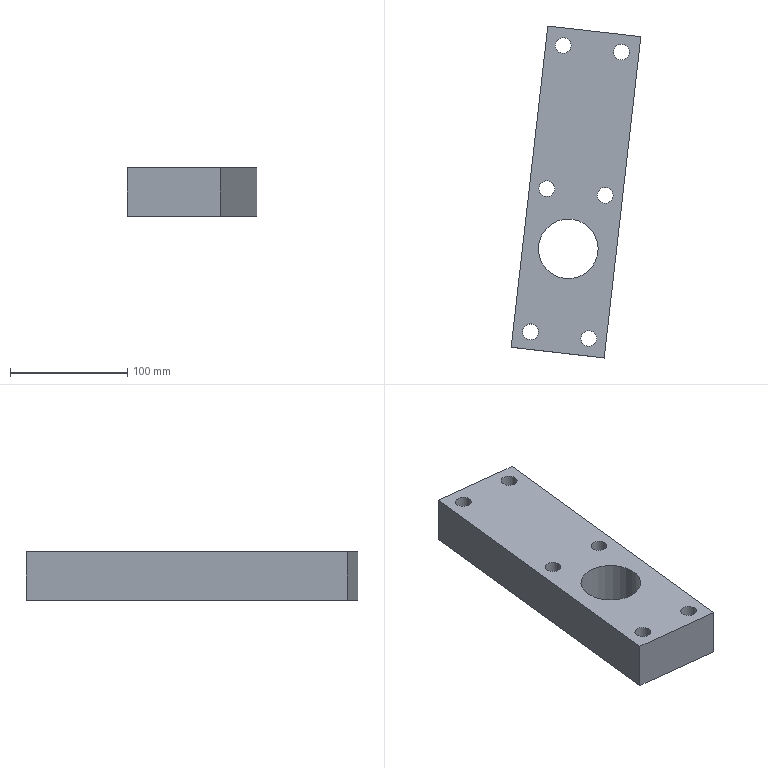Part | NX | features solid 2 | 1 solid | 25 faces | box 110.73 x 283.282 x 41 mm | volume 770920 mm3 | cylinder 13 | plane 12 | commonest cylinder face diameters 13.5 x6 20 x6 51 x1
STEP:
#1=CARTESIAN_POINT('',(2633.711,-284.047,60.));
#2=VERTEX_POINT('',#1);
#3=CARTESIAN_POINT('',(2643.454,-286.297,60.));
#4=DIRECTION('',(0.,0.,-1.));
#5=DIRECTION('',(-0.9744,0.225,0.));
#6=AXIS2_PLACEMENT_3D('',#3,#4,#5);
#7=CIRCLE('',#6,10.);
#8=EDGE_CURVE('',#2,#2,#7,.T.);
#9=ORIENTED_EDGE('',*,*,#8,.F.);
#10=EDGE_LOOP('',(#9));
#11=FACE_BOUND('',#10,.T.);
#12=CARTESIAN_POINT('',(2603.776,-280.637,60.));
#13=VERTEX_POINT('',#12);
#14=CARTESIAN_POINT('',(2593.776,-280.637,60.));
#15=DIRECTION('',(0.,0.,1.));
#16=DIRECTION('',(1.,0.,0.));
#17=AXIS2_PLACEMENT_3D('',#14,#15,#16);
#18=CIRCLE('',#17,10.);
#19=EDGE_CURVE('',#13,#13,#18,.T.);
#20=ORIENTED_EDGE('',*,*,#19,.T.);
#21=EDGE_LOOP('',(#20));
#22=FACE_BOUND('',#21,.T.);
#23=CARTESIAN_POINT('',(2563.25,-416.052,60.));
#24=VERTEX_POINT('',#23);
#25=CARTESIAN_POINT('',(2594.494,-141.826,60.));
#26=VERTEX_POINT('',#25);
#27=CARTESIAN_POINT('',(2579.155,-276.455,60.));
#28=DIRECTION('',(0.1132,0.9936,0.));
#29=VECTOR('',#28,1000.);
#30=LINE('',#27,#29);
#31=EDGE_CURVE('',#24,#26,#30,.T.);
#32=ORIENTED_EDGE('',*,*,#31,.T.);
#33=CARTESIAN_POINT('',(2673.98,-150.882,60.));
#34=VERTEX_POINT('',#33);
#35=CARTESIAN_POINT('',(2673.98,-150.882,60.));
#36=DIRECTION('',(-0.9936,0.1132,0.));
#37=VECTOR('',#36,1000.);
#38=LINE('',#35,#37);
#39=EDGE_CURVE('',#34,#26,#38,.T.);
#40=ORIENTED_EDGE('',*,*,#39,.F.);
#41=CARTESIAN_POINT('',(2642.736,-425.108,60.));
#42=VERTEX_POINT('',#41);
#43=CARTESIAN_POINT('',(2658.641,-285.511,60.));
#44=DIRECTION('',(0.1132,0.9936,0.));
#45=VECTOR('',#44,1000.);
#46=LINE('',#43,#45);
#47=EDGE_CURVE('',#42,#34,#46,.T.);
#48=ORIENTED_EDGE('',*,*,#47,.F.);
#49=CARTESIAN_POINT('',(2642.736,-425.108,60.));
#50=DIRECTION('',(-0.9936,0.1132,0.));
#51=VECTOR('',#50,1000.);
#52=LINE('',#49,#51);
#53=EDGE_CURVE('',#42,#24,#52,.T.);
#54=ORIENTED_EDGE('',*,*,#53,.T.);
#55=EDGE_LOOP('',(#32,#40,#48,#54));
#56=FACE_BOUND('',#55,.T.);
#57=CARTESIAN_POINT('',(2637.5,-332.,60.));
#58=VERTEX_POINT('',#57);
#59=CARTESIAN_POINT('',(2612.,-332.,60.));
#60=DIRECTION('',(0.,0.,-1.));
#61=DIRECTION('',(1.,0.,0.));
#62=AXIS2_PLACEMENT_3D('',#59,#60,#61);
#63=CIRCLE('',#62,25.5);
#64=EDGE_CURVE('',#58,#58,#63,.T.);
#65=ORIENTED_EDGE('',*,*,#64,.F.);
#66=EDGE_LOOP('',(#65));
#67=FACE_BOUND('',#66,.T.);
#68=CARTESIAN_POINT('',(2647.378,-164.088,60.));
#69=VERTEX_POINT('',#68);
#70=CARTESIAN_POINT('',(2657.378,-164.088,60.));
#71=DIRECTION('',(0.,0.,1.));
#72=DIRECTION('',(-1.,0.,0.));
#73=AXIS2_PLACEMENT_3D('',#70,#71,#72);
#74=CIRCLE('',#73,10.);
#75=EDGE_CURVE('',#69,#69,#74,.T.);
#76=ORIENTED_EDGE('',*,*,#75,.T.);
#77=EDGE_LOOP('',(#76));
#78=FACE_BOUND('',#77,.T.);
#79=CARTESIAN_POINT('',(2617.443,-160.677,60.));
#80=VERTEX_POINT('',#79);
#81=CARTESIAN_POINT('',(2607.7,-158.427,60.));
#82=DIRECTION('',(0.,0.,-1.));
#83=DIRECTION('',(0.9744,-0.225,0.));
#84=AXIS2_PLACEMENT_3D('',#81,#82,#83);
#85=CIRCLE('',#84,10.);
#86=EDGE_CURVE('',#80,#80,#85,.T.);
#87=ORIENTED_EDGE('',*,*,#86,.F.);
#88=EDGE_LOOP('',(#87));
#89=FACE_BOUND('',#88,.T.);
#90=CARTESIAN_POINT('',(2589.852,-402.846,60.));
#91=VERTEX_POINT('',#90);
#92=CARTESIAN_POINT('',(2579.852,-402.846,60.));
#93=DIRECTION('',(0.,0.,1.));
#94=DIRECTION('',(1.,0.,0.));
#95=AXIS2_PLACEMENT_3D('',#92,#93,#94);
#96=CIRCLE('',#95,10.);
#97=EDGE_CURVE('',#91,#91,#96,.T.);
#98=ORIENTED_EDGE('',*,*,#97,.T.);
#99=EDGE_LOOP('',(#98));
#100=FACE_BOUND('',#99,.T.);
#101=CARTESIAN_POINT('',(2619.787,-406.257,60.));
#102=VERTEX_POINT('',#101);
#103=CARTESIAN_POINT('',(2629.53,-408.506,60.));
#104=DIRECTION('',(0.,0.,-1.));
#105=DIRECTION('',(-0.9744,0.225,0.));
#106=AXIS2_PLACEMENT_3D('',#103,#104,#105);
#107=CIRCLE('',#106,10.);
#108=EDGE_CURVE('',#102,#102,#107,.T.);
#109=ORIENTED_EDGE('',*,*,#108,.F.);
#110=EDGE_LOOP('',(#109));
#111=FACE_BOUND('',#110,.T.);
#112=CARTESIAN_POINT('',(2658.641,-285.511,60.));
#113=DIRECTION('',(0.,0.,1.));
#114=DIRECTION('',(-1.,0.,0.));
#115=AXIS2_PLACEMENT_3D('',#112,#113,#114);
#116=PLANE('',#115);
#117=ADVANCED_FACE('',(#11,#22,#56,#67,#78,#89,#100,#111),#116,.F.);
#118=CARTESIAN_POINT('',(2622.953,-406.988,101.));
#119=VERTEX_POINT('',#118);
#120=CARTESIAN_POINT('',(2629.53,-408.506,101.));
#121=DIRECTION('',(0.,0.,1.));
#122=DIRECTION('',(-0.9744,0.225,0.));
#123=AXIS2_PLACEMENT_3D('',#120,#121,#122);
#124=CIRCLE('',#123,6.75);
#125=EDGE_CURVE('',#119,#119,#124,.T.);
#126=ORIENTED_EDGE('',*,*,#125,.F.);
#127=EDGE_LOOP('',(#126));
#128=FACE_BOUND('',#127,.T.);
#129=CARTESIAN_POINT('',(2600.526,-280.637,101.));
#130=VERTEX_POINT('',#129);
#131=CARTESIAN_POINT('',(2593.776,-280.637,101.));
#132=DIRECTION('',(0.,0.,-1.));
#133=DIRECTION('',(1.,0.,0.));
#134=AXIS2_PLACEMENT_3D('',#131,#132,#133);
#135=CIRCLE('',#134,6.75);
#136=EDGE_CURVE('',#130,#130,#135,.T.);
#137=ORIENTED_EDGE('',*,*,#136,.T.);
#138=EDGE_LOOP('',(#137));
#139=FACE_BOUND('',#138,.T.);
#140=CARTESIAN_POINT('',(2614.277,-159.946,101.));
#141=VERTEX_POINT('',#140);
#142=CARTESIAN_POINT('',(2607.7,-158.427,101.));
#143=DIRECTION('',(0.,0.,1.));
#144=DIRECTION('',(0.9744,-0.225,0.));
#145=AXIS2_PLACEMENT_3D('',#142,#143,#144);
#146=CIRCLE('',#145,6.75);
#147=EDGE_CURVE('',#141,#141,#146,.T.);
#148=ORIENTED_EDGE('',*,*,#147,.F.);
#149=EDGE_LOOP('',(#148));
#150=FACE_BOUND('',#149,.T.);
#151=CARTESIAN_POINT('',(2637.5,-332.,101.));
#152=VERTEX_POINT('',#151);
#153=CARTESIAN_POINT('',(2612.,-332.,101.));
#154=DIRECTION('',(0.,0.,-1.));
#155=DIRECTION('',(1.,0.,0.));
#156=AXIS2_PLACEMENT_3D('',#153,#154,#155);
#157=CIRCLE('',#156,25.5);
#158=EDGE_CURVE('',#152,#152,#157,.T.);
#159=ORIENTED_EDGE('',*,*,#158,.T.);
#160=EDGE_LOOP('',(#159));
#161=FACE_BOUND('',#160,.T.);
#162=CARTESIAN_POINT('',(2673.98,-150.882,101.));
#163=VERTEX_POINT('',#162);
#164=CARTESIAN_POINT('',(2642.736,-425.108,101.));
#165=VERTEX_POINT('',#164);
#166=CARTESIAN_POINT('',(2658.641,-285.511,101.));
#167=DIRECTION('',(-0.1132,-0.9936,0.));
#168=VECTOR('',#167,1000.);
#169=LINE('',#166,#168);
#170=EDGE_CURVE('',#163,#165,#169,.T.);
#171=ORIENTED_EDGE('',*,*,#170,.F.);
#172=CARTESIAN_POINT('',(2594.494,-141.826,101.));
#173=VERTEX_POINT('',#172);
#174=CARTESIAN_POINT('',(2673.98,-150.882,101.));
#175=DIRECTION('',(-0.9936,0.1132,0.));
#176=VECTOR('',#175,1000.);
#177=LINE('',#174,#176);
#178=EDGE_CURVE('',#163,#173,#177,.T.);
#179=ORIENTED_EDGE('',*,*,#178,.T.);
#180=CARTESIAN_POINT('',(2563.25,-416.052,101.));
#181=VERTEX_POINT('',#180);
#182=CARTESIAN_POINT('',(2579.155,-276.455,101.));
#183=DIRECTION('',(-0.1132,-0.9936,0.));
#184=VECTOR('',#183,1000.);
#185=LINE('',#182,#184);
#186=EDGE_CURVE('',#173,#181,#185,.T.);
#187=ORIENTED_EDGE('',*,*,#186,.T.);
#188=CARTESIAN_POINT('',(2642.736,-425.108,101.));
#189=DIRECTION('',(-0.9936,0.1132,0.));
#190=VECTOR('',#189,1000.);
#191=LINE('',#188,#190);
#192=EDGE_CURVE('',#165,#181,#191,.T.);
#193=ORIENTED_EDGE('',*,*,#192,.F.);
#194=EDGE_LOOP('',(#171,#179,#187,#193));
#195=FACE_BOUND('',#194,.T.);
#196=CARTESIAN_POINT('',(2650.628,-164.088,101.));
#197=VERTEX_POINT('',#196);
#198=CARTESIAN_POINT('',(2657.378,-164.088,101.));
#199=DIRECTION('',(0.,0.,-1.));
#200=DIRECTION('',(-1.,0.,0.));
#201=AXIS2_PLACEMENT_3D('',#198,#199,#200);
#202=CIRCLE('',#201,6.75);
#203=EDGE_CURVE('',#197,#197,#202,.T.);
#204=ORIENTED_EDGE('',*,*,#203,.T.);
#205=EDGE_LOOP('',(#204));
#206=FACE_BOUND('',#205,.T.);
#207=CARTESIAN_POINT('',(2636.877,-284.779,101.));
#208=VERTEX_POINT('',#207);
#209=CARTESIAN_POINT('',(2643.454,-286.297,101.));
#210=DIRECTION('',(0.,0.,1.));
#211=DIRECTION('',(-0.9744,0.225,0.));
#212=AXIS2_PLACEMENT_3D('',#209,#210,#211);
#213=CIRCLE('',#212,6.75);
#214=EDGE_CURVE('',#208,#208,#213,.T.);
#215=ORIENTED_EDGE('',*,*,#214,.F.);
#216=EDGE_LOOP('',(#215));
#217=FACE_BOUND('',#216,.T.);
#218=CARTESIAN_POINT('',(2586.602,-402.846,101.));
#219=VERTEX_POINT('',#218);
#220=CARTESIAN_POINT('',(2579.852,-402.846,101.));
#221=DIRECTION('',(0.,0.,-1.));
#222=DIRECTION('',(1.,0.,0.));
#223=AXIS2_PLACEMENT_3D('',#220,#221,#222);
#224=CIRCLE('',#223,6.75);
#225=EDGE_CURVE('',#219,#219,#224,.T.);
#226=ORIENTED_EDGE('',*,*,#225,.T.);
#227=EDGE_LOOP('',(#226));
#228=FACE_BOUND('',#227,.T.);
#229=CARTESIAN_POINT('',(1945.,0.,101.));
#230=DIRECTION('',(0.,0.,1.));
#231=DIRECTION('',(-1.,0.,0.));
#232=AXIS2_PLACEMENT_3D('',#229,#230,#231);
#233=PLANE('',#232);
#234=ADVANCED_FACE('',(#128,#139,#150,#161,#195,#206,#217,#228),#233,.T.);
#235=ORIENTED_EDGE('',*,*,#178,.F.);
#236=CARTESIAN_POINT('',(2673.98,-150.882,61.));
#237=DIRECTION('',(0.,0.,1.));
#238=VECTOR('',#237,1000.);
#239=LINE('',#236,#238);
#240=EDGE_CURVE('',#34,#163,#239,.T.);
#241=ORIENTED_EDGE('',*,*,#240,.F.);
#242=ORIENTED_EDGE('',*,*,#39,.T.);
#243=CARTESIAN_POINT('',(2594.494,-141.826,61.));
#244=DIRECTION('',(0.,0.,1.));
#245=VECTOR('',#244,1000.);
#246=LINE('',#243,#245);
#247=EDGE_CURVE('',#26,#173,#246,.T.);
#248=ORIENTED_EDGE('',*,*,#247,.T.);
#249=EDGE_LOOP('',(#235,#241,#242,#248));
#250=FACE_BOUND('',#249,.T.);
#251=CARTESIAN_POINT('',(2673.98,-150.882,61.));
#252=DIRECTION('',(-0.1132,-0.9936,0.));
#253=DIRECTION('',(-0.9936,0.1132,0.));
#254=AXIS2_PLACEMENT_3D('',#251,#252,#253);
#255=PLANE('',#254);
#256=ADVANCED_FACE('',(#250),#255,.F.);
#257=CARTESIAN_POINT('',(2642.736,-425.108,61.));
#258=DIRECTION('',(0.,0.,1.));
#259=VECTOR('',#258,1000.);
#260=LINE('',#257,#259);
#261=EDGE_CURVE('',#42,#165,#260,.T.);
#262=ORIENTED_EDGE('',*,*,#261,.T.);
#263=ORIENTED_EDGE('',*,*,#192,.T.);
#264=CARTESIAN_POINT('',(2563.25,-416.052,61.));
#265=DIRECTION('',(0.,0.,1.));
#266=VECTOR('',#265,1000.);
#267=LINE('',#264,#266);
#268=EDGE_CURVE('',#24,#181,#267,.T.);
#269=ORIENTED_EDGE('',*,*,#268,.F.);
#270=ORIENTED_EDGE('',*,*,#53,.F.);
#271=EDGE_LOOP('',(#262,#263,#269,#270));
#272=FACE_BOUND('',#271,.T.);
#273=CARTESIAN_POINT('',(2642.736,-425.108,61.));
#274=DIRECTION('',(-0.1132,-0.9936,0.));
#275=DIRECTION('',(-0.9936,0.1132,0.));
#276=AXIS2_PLACEMENT_3D('',#273,#274,#275);
#277=PLANE('',#276);
#278=ADVANCED_FACE('',(#272),#277,.T.);
#279=ORIENTED_EDGE('',*,*,#240,.T.);
#280=ORIENTED_EDGE('',*,*,#170,.T.);
#281=ORIENTED_EDGE('',*,*,#261,.F.);
#282=ORIENTED_EDGE('',*,*,#47,.T.);
#283=EDGE_LOOP('',(#279,#280,#281,#282));
#284=FACE_BOUND('',#283,.T.);
#285=CARTESIAN_POINT('',(2658.641,-285.511,61.));
#286=DIRECTION('',(0.9936,-0.1132,0.));
#287=DIRECTION('',(0.,0.,1.));
#288=AXIS2_PLACEMENT_3D('',#285,#286,#287);
#289=PLANE('',#288);
#290=ADVANCED_FACE('',(#284),#289,.T.);
#291=ORIENTED_EDGE('',*,*,#186,.F.);
#292=ORIENTED_EDGE('',*,*,#247,.F.);
#293=ORIENTED_EDGE('',*,*,#31,.F.);
#294=ORIENTED_EDGE('',*,*,#268,.T.);
#295=EDGE_LOOP('',(#291,#292,#293,#294));
#296=FACE_BOUND('',#295,.T.);
#297=CARTESIAN_POINT('',(2579.155,-276.455,61.));
#298=DIRECTION('',(0.9936,-0.1132,0.));
#299=DIRECTION('',(0.,0.,1.));
#300=AXIS2_PLACEMENT_3D('',#297,#298,#299);
#301=PLANE('',#300);
#302=ADVANCED_FACE('',(#296),#301,.F.);
#303=ORIENTED_EDGE('',*,*,#64,.T.);
#304=EDGE_LOOP('',(#303));
#305=FACE_BOUND('',#304,.T.);
#306=ORIENTED_EDGE('',*,*,#158,.F.);
#307=EDGE_LOOP('',(#306));
#308=FACE_BOUND('',#307,.T.);
#309=CARTESIAN_POINT('',(2612.,-332.,-101.));
#310=DIRECTION('',(0.,0.,1.));
#311=DIRECTION('',(-1.,0.,0.));
#312=AXIS2_PLACEMENT_3D('',#309,#310,#311);
#313=CYLINDRICAL_SURFACE('',#312,25.5);
#314=ADVANCED_FACE('',(#305,#308),#313,.F.);
#315=CARTESIAN_POINT('',(2650.628,-164.088,75.));
#316=VERTEX_POINT('',#315);
#317=CARTESIAN_POINT('',(2657.378,-164.088,75.));
#318=DIRECTION('',(0.,0.,1.));
#319=DIRECTION('',(-1.,0.,0.));
#320=AXIS2_PLACEMENT_3D('',#317,#318,#319);
#321=CIRCLE('',#320,6.75);
#322=EDGE_CURVE('',#316,#316,#321,.T.);
#323=ORIENTED_EDGE('',*,*,#322,.F.);
#324=EDGE_LOOP('',(#323));
#325=FACE_BOUND('',#324,.T.);
#326=ORIENTED_EDGE('',*,*,#203,.F.);
#327=EDGE_LOOP('',(#326));
#328=FACE_BOUND('',#327,.T.);
#329=CARTESIAN_POINT('',(2657.378,-164.088,60.));
#330=DIRECTION('',(0.,0.,1.));
#331=DIRECTION('',(1.,0.,0.));
#332=AXIS2_PLACEMENT_3D('',#329,#330,#331);
#333=CYLINDRICAL_SURFACE('',#332,6.75);
#334=ADVANCED_FACE('',(#325,#328),#333,.F.);
#335=ORIENTED_EDGE('',*,*,#322,.T.);
#336=EDGE_LOOP('',(#335));
#337=FACE_BOUND('',#336,.T.);
#338=CARTESIAN_POINT('',(2647.378,-164.088,75.));
#339=VERTEX_POINT('',#338);
#340=CARTESIAN_POINT('',(2657.378,-164.088,75.));
#341=DIRECTION('',(0.,0.,1.));
#342=DIRECTION('',(-1.,0.,0.));
#343=AXIS2_PLACEMENT_3D('',#340,#341,#342);
#344=CIRCLE('',#343,10.);
#345=EDGE_CURVE('',#339,#339,#344,.T.);
#346=ORIENTED_EDGE('',*,*,#345,.F.);
#347=EDGE_LOOP('',(#346));
#348=FACE_BOUND('',#347,.T.);
#349=CARTESIAN_POINT('',(2657.378,-164.088,75.));
#350=DIRECTION('',(0.,0.,1.));
#351=DIRECTION('',(1.,0.,0.));
#352=AXIS2_PLACEMENT_3D('',#349,#350,#351);
#353=PLANE('',#352);
#354=ADVANCED_FACE('',(#337,#348),#353,.F.);
#355=ORIENTED_EDGE('',*,*,#345,.T.);
#356=EDGE_LOOP('',(#355));
#357=FACE_BOUND('',#356,.T.);
#358=ORIENTED_EDGE('',*,*,#75,.F.);
#359=EDGE_LOOP('',(#358));
#360=FACE_BOUND('',#359,.T.);
#361=CARTESIAN_POINT('',(2657.378,-164.088,60.));
#362=DIRECTION('',(0.,0.,1.));
#363=DIRECTION('',(1.,0.,0.));
#364=AXIS2_PLACEMENT_3D('',#361,#362,#363);
#365=CYLINDRICAL_SURFACE('',#364,10.);
#366=ADVANCED_FACE('',(#357,#360),#365,.F.);
#367=CARTESIAN_POINT('',(2614.277,-159.946,75.));
#368=VERTEX_POINT('',#367);
#369=CARTESIAN_POINT('',(2607.7,-158.427,75.));
#370=DIRECTION('',(0.,0.,-1.));
#371=DIRECTION('',(0.9744,-0.225,0.));
#372=AXIS2_PLACEMENT_3D('',#369,#370,#371);
#373=CIRCLE('',#372,6.75);
#374=EDGE_CURVE('',#368,#368,#373,.T.);
#375=ORIENTED_EDGE('',*,*,#374,.T.);
#376=EDGE_LOOP('',(#375));
#377=FACE_BOUND('',#376,.T.);
#378=ORIENTED_EDGE('',*,*,#147,.T.);
#379=EDGE_LOOP('',(#378));
#380=FACE_BOUND('',#379,.T.);
#381=CARTESIAN_POINT('',(2607.7,-158.427,60.));
#382=DIRECTION('',(0.,0.,1.));
#383=DIRECTION('',(-0.9744,0.225,0.));
#384=AXIS2_PLACEMENT_3D('',#381,#382,#383);
#385=CYLINDRICAL_SURFACE('',#384,6.75);
#386=ADVANCED_FACE('',(#377,#380),#385,.F.);
#387=ORIENTED_EDGE('',*,*,#374,.F.);
#388=EDGE_LOOP('',(#387));
#389=FACE_BOUND('',#388,.T.);
#390=CARTESIAN_POINT('',(2617.443,-160.677,75.));
#391=VERTEX_POINT('',#390);
#392=CARTESIAN_POINT('',(2607.7,-158.427,75.));
#393=DIRECTION('',(0.,0.,-1.));
#394=DIRECTION('',(0.9744,-0.225,0.));
#395=AXIS2_PLACEMENT_3D('',#392,#393,#394);
#396=CIRCLE('',#395,10.);
#397=EDGE_CURVE('',#391,#391,#396,.T.);
#398=ORIENTED_EDGE('',*,*,#397,.T.);
#399=EDGE_LOOP('',(#398));
#400=FACE_BOUND('',#399,.T.);
#401=CARTESIAN_POINT('',(2607.7,-158.427,75.));
#402=DIRECTION('',(0.,0.,1.));
#403=DIRECTION('',(-0.9744,0.225,0.));
#404=AXIS2_PLACEMENT_3D('',#401,#402,#403);
#405=PLANE('',#404);
#406=ADVANCED_FACE('',(#389,#400),#405,.F.);
#407=ORIENTED_EDGE('',*,*,#397,.F.);
#408=EDGE_LOOP('',(#407));
#409=FACE_BOUND('',#408,.T.);
#410=ORIENTED_EDGE('',*,*,#86,.T.);
#411=EDGE_LOOP('',(#410));
#412=FACE_BOUND('',#411,.T.);
#413=CARTESIAN_POINT('',(2607.7,-158.427,60.));
#414=DIRECTION('',(0.,0.,1.));
#415=DIRECTION('',(-0.9744,0.225,0.));
#416=AXIS2_PLACEMENT_3D('',#413,#414,#415);
#417=CYLINDRICAL_SURFACE('',#416,10.);
#418=ADVANCED_FACE('',(#409,#412),#417,.F.);
#419=CARTESIAN_POINT('',(2600.526,-280.637,75.));
#420=VERTEX_POINT('',#419);
#421=CARTESIAN_POINT('',(2593.776,-280.637,75.));
#422=DIRECTION('',(0.,0.,1.));
#423=DIRECTION('',(1.,0.,0.));
#424=AXIS2_PLACEMENT_3D('',#421,#422,#423);
#425=CIRCLE('',#424,6.75);
#426=EDGE_CURVE('',#420,#420,#425,.T.);
#427=ORIENTED_EDGE('',*,*,#426,.F.);
#428=EDGE_LOOP('',(#427));
#429=FACE_BOUND('',#428,.T.);
#430=ORIENTED_EDGE('',*,*,#136,.F.);
#431=EDGE_LOOP('',(#430));
#432=FACE_BOUND('',#431,.T.);
#433=CARTESIAN_POINT('',(2593.776,-280.637,60.));
#434=DIRECTION('',(0.,0.,1.));
#435=DIRECTION('',(-1.,0.,0.));
#436=AXIS2_PLACEMENT_3D('',#433,#434,#435);
#437=CYLINDRICAL_SURFACE('',#436,6.75);
#438=ADVANCED_FACE('',(#429,#432),#437,.F.);
#439=ORIENTED_EDGE('',*,*,#426,.T.);
#440=EDGE_LOOP('',(#439));
#441=FACE_BOUND('',#440,.T.);
#442=CARTESIAN_POINT('',(2603.776,-280.637,75.));
#443=VERTEX_POINT('',#442);
#444=CARTESIAN_POINT('',(2593.776,-280.637,75.));
#445=DIRECTION('',(0.,0.,1.));
#446=DIRECTION('',(1.,0.,0.));
#447=AXIS2_PLACEMENT_3D('',#444,#445,#446);
#448=CIRCLE('',#447,10.);
#449=EDGE_CURVE('',#443,#443,#448,.T.);
#450=ORIENTED_EDGE('',*,*,#449,.F.);
#451=EDGE_LOOP('',(#450));
#452=FACE_BOUND('',#451,.T.);
#453=CARTESIAN_POINT('',(2593.776,-280.637,75.));
#454=DIRECTION('',(0.,0.,1.));
#455=DIRECTION('',(-1.,0.,0.));
#456=AXIS2_PLACEMENT_3D('',#453,#454,#455);
#457=PLANE('',#456);
#458=ADVANCED_FACE('',(#441,#452),#457,.F.);
#459=ORIENTED_EDGE('',*,*,#449,.T.);
#460=EDGE_LOOP('',(#459));
#461=FACE_BOUND('',#460,.T.);
#462=ORIENTED_EDGE('',*,*,#19,.F.);
#463=EDGE_LOOP('',(#462));
#464=FACE_BOUND('',#463,.T.);
#465=CARTESIAN_POINT('',(2593.776,-280.637,60.));
#466=DIRECTION('',(0.,0.,1.));
#467=DIRECTION('',(-1.,0.,0.));
#468=AXIS2_PLACEMENT_3D('',#465,#466,#467);
#469=CYLINDRICAL_SURFACE('',#468,10.);
#470=ADVANCED_FACE('',(#461,#464),#469,.F.);
#471=CARTESIAN_POINT('',(2636.877,-284.779,75.));
#472=VERTEX_POINT('',#471);
#473=CARTESIAN_POINT('',(2643.454,-286.297,75.));
#474=DIRECTION('',(0.,0.,-1.));
#475=DIRECTION('',(-0.9744,0.225,0.));
#476=AXIS2_PLACEMENT_3D('',#473,#474,#475);
#477=CIRCLE('',#476,6.75);
#478=EDGE_CURVE('',#472,#472,#477,.T.);
#479=ORIENTED_EDGE('',*,*,#478,.T.);
#480=EDGE_LOOP('',(#479));
#481=FACE_BOUND('',#480,.T.);
#482=ORIENTED_EDGE('',*,*,#214,.T.);
#483=EDGE_LOOP('',(#482));
#484=FACE_BOUND('',#483,.T.);
#485=CARTESIAN_POINT('',(2643.454,-286.297,60.));
#486=DIRECTION('',(0.,0.,1.));
#487=DIRECTION('',(0.9744,-0.225,0.));
#488=AXIS2_PLACEMENT_3D('',#485,#486,#487);
#489=CYLINDRICAL_SURFACE('',#488,6.75);
#490=ADVANCED_FACE('',(#481,#484),#489,.F.);
#491=ORIENTED_EDGE('',*,*,#478,.F.);
#492=EDGE_LOOP('',(#491));
#493=FACE_BOUND('',#492,.T.);
#494=CARTESIAN_POINT('',(2633.711,-284.047,75.));
#495=VERTEX_POINT('',#494);
#496=CARTESIAN_POINT('',(2643.454,-286.297,75.));
#497=DIRECTION('',(0.,0.,-1.));
#498=DIRECTION('',(-0.9744,0.225,0.));
#499=AXIS2_PLACEMENT_3D('',#496,#497,#498);
#500=CIRCLE('',#499,10.);
#501=EDGE_CURVE('',#495,#495,#500,.T.);
#502=ORIENTED_EDGE('',*,*,#501,.T.);
#503=EDGE_LOOP('',(#502));
#504=FACE_BOUND('',#503,.T.);
#505=CARTESIAN_POINT('',(2643.454,-286.297,75.));
#506=DIRECTION('',(0.,0.,1.));
#507=DIRECTION('',(0.9744,-0.225,0.));
#508=AXIS2_PLACEMENT_3D('',#505,#506,#507);
#509=PLANE('',#508);
#510=ADVANCED_FACE('',(#493,#504),#509,.F.);
#511=ORIENTED_EDGE('',*,*,#501,.F.);
#512=EDGE_LOOP('',(#511));
#513=FACE_BOUND('',#512,.T.);
#514=ORIENTED_EDGE('',*,*,#8,.T.);
#515=EDGE_LOOP('',(#514));
#516=FACE_BOUND('',#515,.T.);
#517=CARTESIAN_POINT('',(2643.454,-286.297,60.));
#518=DIRECTION('',(0.,0.,1.));
#519=DIRECTION('',(0.9744,-0.225,0.));
#520=AXIS2_PLACEMENT_3D('',#517,#518,#519);
#521=CYLINDRICAL_SURFACE('',#520,10.);
#522=ADVANCED_FACE('',(#513,#516),#521,.F.);
#523=CARTESIAN_POINT('',(2586.602,-402.846,75.));
#524=VERTEX_POINT('',#523);
#525=CARTESIAN_POINT('',(2579.852,-402.846,75.));
#526=DIRECTION('',(0.,0.,1.));
#527=DIRECTION('',(1.,0.,0.));
#528=AXIS2_PLACEMENT_3D('',#525,#526,#527);
#529=CIRCLE('',#528,6.75);
#530=EDGE_CURVE('',#524,#524,#529,.T.);
#531=ORIENTED_EDGE('',*,*,#530,.F.);
#532=EDGE_LOOP('',(#531));
#533=FACE_BOUND('',#532,.T.);
#534=ORIENTED_EDGE('',*,*,#225,.F.);
#535=EDGE_LOOP('',(#534));
#536=FACE_BOUND('',#535,.T.);
#537=CARTESIAN_POINT('',(2579.852,-402.846,60.));
#538=DIRECTION('',(0.,0.,1.));
#539=DIRECTION('',(-1.,0.,0.));
#540=AXIS2_PLACEMENT_3D('',#537,#538,#539);
#541=CYLINDRICAL_SURFACE('',#540,6.75);
#542=ADVANCED_FACE('',(#533,#536),#541,.F.);
#543=ORIENTED_EDGE('',*,*,#530,.T.);
#544=EDGE_LOOP('',(#543));
#545=FACE_BOUND('',#544,.T.);
#546=CARTESIAN_POINT('',(2589.852,-402.846,75.));
#547=VERTEX_POINT('',#546);
#548=CARTESIAN_POINT('',(2579.852,-402.846,75.));
#549=DIRECTION('',(0.,0.,1.));
#550=DIRECTION('',(1.,0.,0.));
#551=AXIS2_PLACEMENT_3D('',#548,#549,#550);
#552=CIRCLE('',#551,10.);
#553=EDGE_CURVE('',#547,#547,#552,.T.);
#554=ORIENTED_EDGE('',*,*,#553,.F.);
#555=EDGE_LOOP('',(#554));
#556=FACE_BOUND('',#555,.T.);
#557=CARTESIAN_POINT('',(2579.852,-402.846,75.));
#558=DIRECTION('',(0.,0.,1.));
#559=DIRECTION('',(-1.,0.,0.));
#560=AXIS2_PLACEMENT_3D('',#557,#558,#559);
#561=PLANE('',#560);
#562=ADVANCED_FACE('',(#545,#556),#561,.F.);
#563=ORIENTED_EDGE('',*,*,#553,.T.);
#564=EDGE_LOOP('',(#563));
#565=FACE_BOUND('',#564,.T.);
#566=ORIENTED_EDGE('',*,*,#97,.F.);
#567=EDGE_LOOP('',(#566));
#568=FACE_BOUND('',#567,.T.);
#569=CARTESIAN_POINT('',(2579.852,-402.846,60.));
#570=DIRECTION('',(0.,0.,1.));
#571=DIRECTION('',(-1.,0.,0.));
#572=AXIS2_PLACEMENT_3D('',#569,#570,#571);
#573=CYLINDRICAL_SURFACE('',#572,10.);
#574=ADVANCED_FACE('',(#565,#568),#573,.F.);
#575=CARTESIAN_POINT('',(2622.953,-406.988,75.));
#576=VERTEX_POINT('',#575);
#577=CARTESIAN_POINT('',(2629.53,-408.506,75.));
#578=DIRECTION('',(0.,0.,-1.));
#579=DIRECTION('',(-0.9744,0.225,0.));
#580=AXIS2_PLACEMENT_3D('',#577,#578,#579);
#581=CIRCLE('',#580,6.75);
#582=EDGE_CURVE('',#576,#576,#581,.T.);
#583=ORIENTED_EDGE('',*,*,#582,.T.);
#584=EDGE_LOOP('',(#583));
#585=FACE_BOUND('',#584,.T.);
#586=ORIENTED_EDGE('',*,*,#125,.T.);
#587=EDGE_LOOP('',(#586));
#588=FACE_BOUND('',#587,.T.);
#589=CARTESIAN_POINT('',(2629.53,-408.506,60.));
#590=DIRECTION('',(0.,0.,1.));
#591=DIRECTION('',(0.9744,-0.225,0.));
#592=AXIS2_PLACEMENT_3D('',#589,#590,#591);
#593=CYLINDRICAL_SURFACE('',#592,6.75);
#594=ADVANCED_FACE('',(#585,#588),#593,.F.);
#595=ORIENTED_EDGE('',*,*,#582,.F.);
#596=EDGE_LOOP('',(#595));
#597=FACE_BOUND('',#596,.T.);
#598=CARTESIAN_POINT('',(2619.787,-406.257,75.));
#599=VERTEX_POINT('',#598);
#600=CARTESIAN_POINT('',(2629.53,-408.506,75.));
#601=DIRECTION('',(0.,0.,-1.));
#602=DIRECTION('',(-0.9744,0.225,0.));
#603=AXIS2_PLACEMENT_3D('',#600,#601,#602);
#604=CIRCLE('',#603,10.);
#605=EDGE_CURVE('',#599,#599,#604,.T.);
#606=ORIENTED_EDGE('',*,*,#605,.T.);
#607=EDGE_LOOP('',(#606));
#608=FACE_BOUND('',#607,.T.);
#609=CARTESIAN_POINT('',(2629.53,-408.506,75.));
#610=DIRECTION('',(0.,0.,1.));
#611=DIRECTION('',(0.9744,-0.225,0.));
#612=AXIS2_PLACEMENT_3D('',#609,#610,#611);
#613=PLANE('',#612);
#614=ADVANCED_FACE('',(#597,#608),#613,.F.);
#615=ORIENTED_EDGE('',*,*,#605,.F.);
#616=EDGE_LOOP('',(#615));
#617=FACE_BOUND('',#616,.T.);
#618=ORIENTED_EDGE('',*,*,#108,.T.);
#619=EDGE_LOOP('',(#618));
#620=FACE_BOUND('',#619,.T.);
#621=CARTESIAN_POINT('',(2629.53,-408.506,60.));
#622=DIRECTION('',(0.,0.,1.));
#623=DIRECTION('',(0.9744,-0.225,0.));
#624=AXIS2_PLACEMENT_3D('',#621,#622,#623);
#625=CYLINDRICAL_SURFACE('',#624,10.);
#626=ADVANCED_FACE('',(#617,#620),#625,.F.);
#627=CLOSED_SHELL('',(#117,#234,#256,#278,#290,#302,#314,#334,#354,#366,#386,#406,#418,#438,#458,#470,#490,#510,#522,#542,#562,#574,#594,#614,#626));
#628=MANIFOLD_SOLID_BREP('',#627);
#629=(LENGTH_UNIT()NAMED_UNIT(*)SI_UNIT(.MILLI.,.METRE.));
#630=UNCERTAINTY_MEASURE_WITH_UNIT(LENGTH_MEASURE(0.00001),#629,'','');
#631=(NAMED_UNIT(*)PLANE_ANGLE_UNIT()SI_UNIT($,.RADIAN.));
#632=(NAMED_UNIT(*)SI_UNIT($,.STERADIAN.)SOLID_ANGLE_UNIT());
#633=(GEOMETRIC_REPRESENTATION_CONTEXT(3)GLOBAL_UNCERTAINTY_ASSIGNED_CONTEXT((#630))GLOBAL_UNIT_ASSIGNED_CONTEXT((#629,#631,#632))REPRESENTATION_CONTEXT('',''));
#634=ADVANCED_BREP_SHAPE_REPRESENTATION('',(#628),#633);